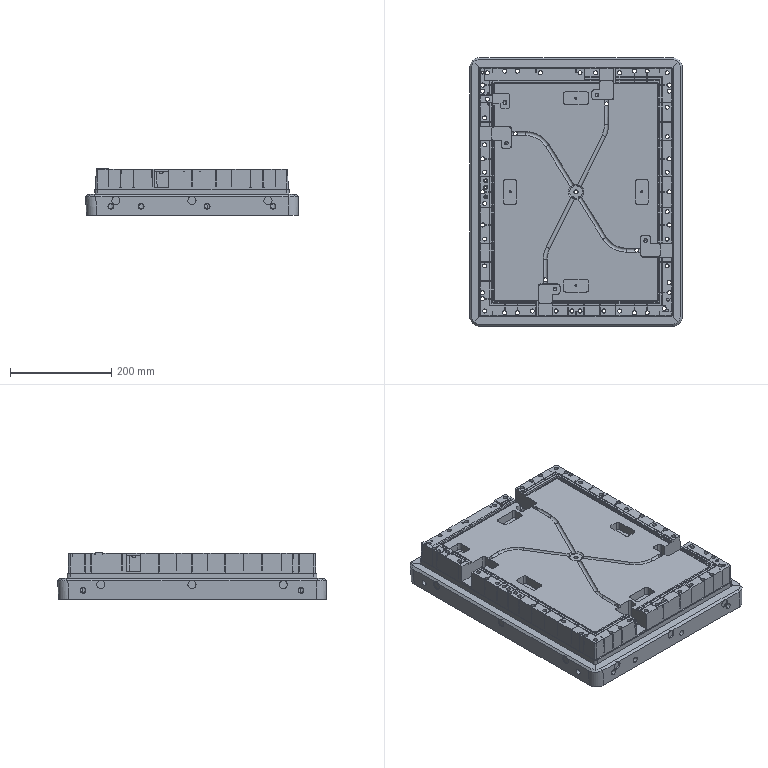Part | Creo | 1 solid | 1771 faces | box 419.84 x 529.844 x 91.787 mm | volume 15998723 mm3 | plane 891 | cylinder 629 | cone 168 | other 61 | torus 12 | spline 6 | sphere 4 | commonest cylinder face diameters 10 x156 8 x129 16 x109 8.032 x44 10.199 x40 10.2 x40